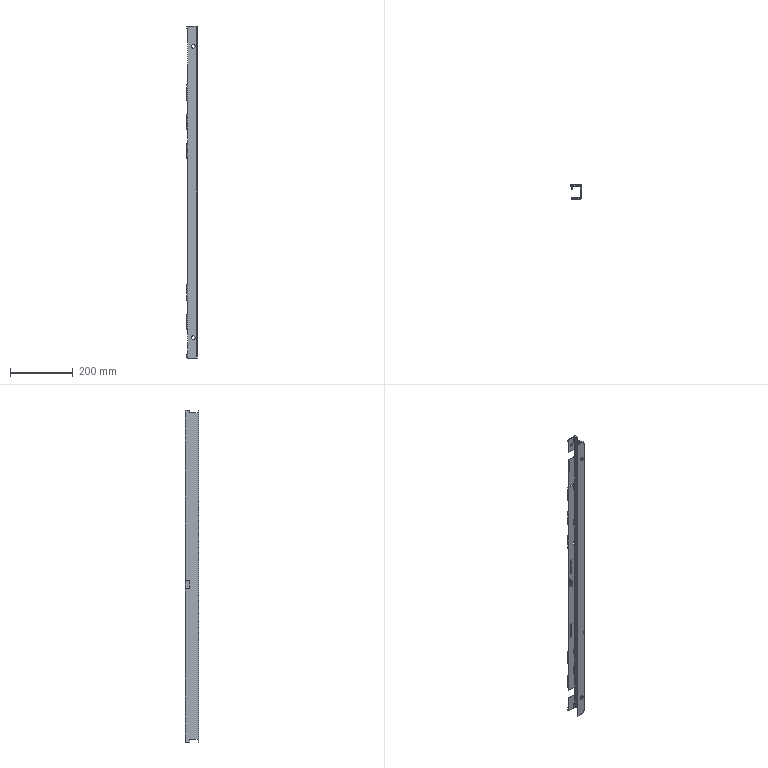Part | NX | features solid 2 | 1 solid | 193 faces | box 32.003 x 43.207 x 1061 mm | volume 200760 mm3 | plane 171 | cylinder 20 | spline 2 | commonest cylinder face diameters 4.004 x10 12 x4 2 x2 6 x2 0.6 x1 4.6 x1